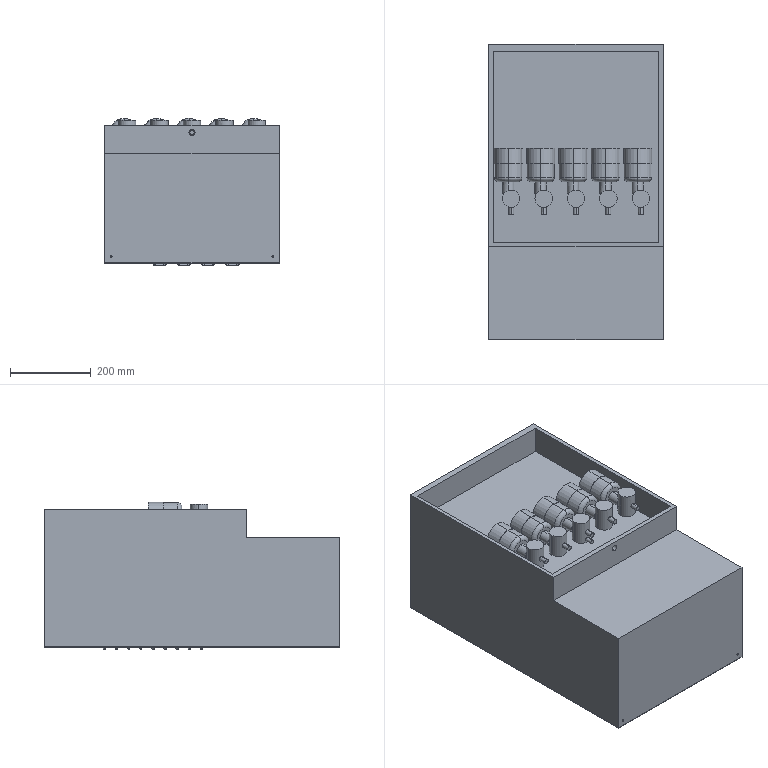Part | STEP file | Beverage coffee machine V1.201001 | 9 solids | 783 faces | box 430 x 730 x 364 mm | volume 89425555 mm3 | cylinder 338 | torus 158 | sphere 144 | plane 143 | commonest cylinder face diameters 12 x50 2 x36 4 x36 12.625 x36 14 x36 102.068 x28